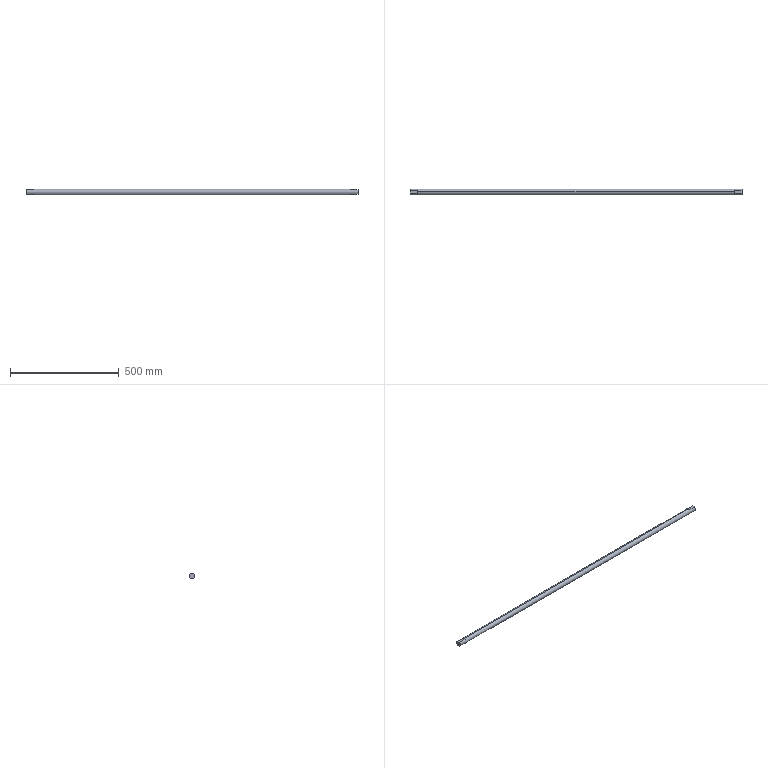Part | SolidWorks | features ICE 3, Extrusion 1, HoleWzd 1 | 1 solid | 12 faces | box 1530 x 25 x 25 mm | volume 749305 mm3 | plane 10 | cylinder 2 | commonest cylinder face diameters 25 x2
STEP:
#1=CARTESIAN_POINT('',(1494.,5.937,-11.));
#2=VERTEX_POINT('',#1);
#3=CARTESIAN_POINT('',(1494.,0.,-12.5));
#4=VERTEX_POINT('',#3);
#5=CARTESIAN_POINT('',(1494.,0.,0.));
#6=DIRECTION('',(-1.,0.,0.));
#7=DIRECTION('',(0.,0.,1.));
#8=AXIS2_PLACEMENT_3D('',#5,#6,#7);
#9=CIRCLE('',#8,12.5);
#10=EDGE_CURVE('',#2,#4,#9,.T.);
#11=ORIENTED_EDGE('',*,*,#10,.T.);
#12=CARTESIAN_POINT('',(36.,0.,-12.5));
#13=VERTEX_POINT('',#12);
#14=CARTESIAN_POINT('',(1530.,0.,-12.5));
#15=DIRECTION('',(-1.,0.,0.));
#16=VECTOR('',#15,1000.);
#17=LINE('',#14,#16);
#18=EDGE_CURVE('',#4,#13,#17,.T.);
#19=ORIENTED_EDGE('',*,*,#18,.T.);
#20=CARTESIAN_POINT('',(36.,5.937,-11.));
#21=VERTEX_POINT('',#20);
#22=CARTESIAN_POINT('',(36.,0.,0.));
#23=DIRECTION('',(1.,0.,0.));
#24=DIRECTION('',(0.,1.,0.));
#25=AXIS2_PLACEMENT_3D('',#22,#23,#24);
#26=CIRCLE('',#25,12.5);
#27=EDGE_CURVE('',#13,#21,#26,.T.);
#28=ORIENTED_EDGE('',*,*,#27,.T.);
#29=CARTESIAN_POINT('',(0.,5.937,-11.));
#30=VERTEX_POINT('',#29);
#31=CARTESIAN_POINT('',(1530.,5.937,-11.));
#32=DIRECTION('',(-1.,0.,0.));
#33=VECTOR('',#32,1000.);
#34=LINE('',#31,#33);
#35=EDGE_CURVE('',#21,#30,#34,.T.);
#36=ORIENTED_EDGE('',*,*,#35,.T.);
#37=CARTESIAN_POINT('',(0.,5.937,11.));
#38=VERTEX_POINT('',#37);
#39=CARTESIAN_POINT('',(0.,0.,0.));
#40=DIRECTION('',(1.,0.,0.));
#41=DIRECTION('',(0.,0.,-1.));
#42=AXIS2_PLACEMENT_3D('',#39,#40,#41);
#43=CIRCLE('',#42,12.5);
#44=EDGE_CURVE('',#30,#38,#43,.T.);
#45=ORIENTED_EDGE('',*,*,#44,.T.);
#46=CARTESIAN_POINT('',(36.,5.937,11.));
#47=VERTEX_POINT('',#46);
#48=CARTESIAN_POINT('',(1530.,5.937,11.));
#49=DIRECTION('',(-1.,0.,0.));
#50=VECTOR('',#49,1000.);
#51=LINE('',#48,#50);
#52=EDGE_CURVE('',#47,#38,#51,.T.);
#53=ORIENTED_EDGE('',*,*,#52,.F.);
#54=CARTESIAN_POINT('',(36.,0.,12.5));
#55=VERTEX_POINT('',#54);
#56=CARTESIAN_POINT('',(36.,0.,0.));
#57=DIRECTION('',(-1.,0.,0.));
#58=DIRECTION('',(0.,-1.,0.));
#59=AXIS2_PLACEMENT_3D('',#56,#57,#58);
#60=CIRCLE('',#59,12.5);
#61=EDGE_CURVE('',#55,#47,#60,.T.);
#62=ORIENTED_EDGE('',*,*,#61,.F.);
#63=CARTESIAN_POINT('',(1494.,0.,12.5));
#64=VERTEX_POINT('',#63);
#65=CARTESIAN_POINT('',(1530.,0.,12.5));
#66=DIRECTION('',(-1.,0.,0.));
#67=VECTOR('',#66,1000.);
#68=LINE('',#65,#67);
#69=EDGE_CURVE('',#64,#55,#68,.T.);
#70=ORIENTED_EDGE('',*,*,#69,.F.);
#71=CARTESIAN_POINT('',(1494.,5.937,11.));
#72=VERTEX_POINT('',#71);
#73=CARTESIAN_POINT('',(1494.,0.,0.));
#74=DIRECTION('',(1.,0.,0.));
#75=DIRECTION('',(0.,0.,-1.));
#76=AXIS2_PLACEMENT_3D('',#73,#74,#75);
#77=CIRCLE('',#76,12.5);
#78=EDGE_CURVE('',#72,#64,#77,.T.);
#79=ORIENTED_EDGE('',*,*,#78,.F.);
#80=CARTESIAN_POINT('',(1530.,5.937,11.));
#81=VERTEX_POINT('',#80);
#82=CARTESIAN_POINT('',(1530.,5.937,11.));
#83=DIRECTION('',(-1.,0.,0.));
#84=VECTOR('',#83,1000.);
#85=LINE('',#82,#84);
#86=EDGE_CURVE('',#81,#72,#85,.T.);
#87=ORIENTED_EDGE('',*,*,#86,.F.);
#88=CARTESIAN_POINT('',(1530.,5.937,-11.));
#89=VERTEX_POINT('',#88);
#90=CARTESIAN_POINT('',(1530.,0.,0.));
#91=DIRECTION('',(1.,0.,0.));
#92=DIRECTION('',(0.,0.,-1.));
#93=AXIS2_PLACEMENT_3D('',#90,#91,#92);
#94=CIRCLE('',#93,12.5);
#95=EDGE_CURVE('',#89,#81,#94,.T.);
#96=ORIENTED_EDGE('',*,*,#95,.F.);
#97=CARTESIAN_POINT('',(1530.,5.937,-11.));
#98=DIRECTION('',(-1.,0.,0.));
#99=VECTOR('',#98,1000.);
#100=LINE('',#97,#99);
#101=EDGE_CURVE('',#89,#2,#100,.T.);
#102=ORIENTED_EDGE('',*,*,#101,.T.);
#103=EDGE_LOOP('',(#11,#19,#28,#36,#45,#53,#62,#70,#79,#87,#96,#102));
#104=FACE_OUTER_BOUND('',#103,.T.);
#105=CARTESIAN_POINT('',(1530.,0.,0.));
#106=DIRECTION('',(-1.,0.,0.));
#107=DIRECTION('',(0.,0.,1.));
#108=AXIS2_PLACEMENT_3D('',#105,#106,#107);
#109=CYLINDRICAL_SURFACE('',#108,12.5);
#110=ADVANCED_FACE('',(#104),#109,.T.);
#111=ORIENTED_EDGE('',*,*,#18,.F.);
#112=CARTESIAN_POINT('',(1494.,-5.937,-11.));
#113=VERTEX_POINT('',#112);
#114=CARTESIAN_POINT('',(1494.,0.,0.));
#115=DIRECTION('',(-1.,0.,0.));
#116=DIRECTION('',(0.,0.,1.));
#117=AXIS2_PLACEMENT_3D('',#114,#115,#116);
#118=CIRCLE('',#117,12.5);
#119=EDGE_CURVE('',#4,#113,#118,.T.);
#120=ORIENTED_EDGE('',*,*,#119,.T.);
#121=CARTESIAN_POINT('',(1530.,-5.937,-11.));
#122=VERTEX_POINT('',#121);
#123=CARTESIAN_POINT('',(1530.,-5.937,-11.));
#124=DIRECTION('',(1.,0.,0.));
#125=VECTOR('',#124,1000.);
#126=LINE('',#123,#125);
#127=EDGE_CURVE('',#113,#122,#126,.T.);
#128=ORIENTED_EDGE('',*,*,#127,.T.);
#129=CARTESIAN_POINT('',(1530.,-5.937,11.));
#130=VERTEX_POINT('',#129);
#131=CARTESIAN_POINT('',(1530.,0.,0.));
#132=DIRECTION('',(1.,0.,0.));
#133=DIRECTION('',(0.,0.,-1.));
#134=AXIS2_PLACEMENT_3D('',#131,#132,#133);
#135=CIRCLE('',#134,12.5);
#136=EDGE_CURVE('',#130,#122,#135,.T.);
#137=ORIENTED_EDGE('',*,*,#136,.F.);
#138=CARTESIAN_POINT('',(1494.,-5.937,11.));
#139=VERTEX_POINT('',#138);
#140=CARTESIAN_POINT('',(1530.,-5.937,11.));
#141=DIRECTION('',(1.,0.,0.));
#142=VECTOR('',#141,1000.);
#143=LINE('',#140,#142);
#144=EDGE_CURVE('',#139,#130,#143,.T.);
#145=ORIENTED_EDGE('',*,*,#144,.F.);
#146=CARTESIAN_POINT('',(1494.,0.,0.));
#147=DIRECTION('',(1.,0.,0.));
#148=DIRECTION('',(0.,0.,-1.));
#149=AXIS2_PLACEMENT_3D('',#146,#147,#148);
#150=CIRCLE('',#149,12.5);
#151=EDGE_CURVE('',#64,#139,#150,.T.);
#152=ORIENTED_EDGE('',*,*,#151,.F.);
#153=ORIENTED_EDGE('',*,*,#69,.T.);
#154=CARTESIAN_POINT('',(36.,-5.937,11.));
#155=VERTEX_POINT('',#154);
#156=CARTESIAN_POINT('',(36.,0.,0.));
#157=DIRECTION('',(-1.,0.,0.));
#158=DIRECTION('',(0.,-1.,0.));
#159=AXIS2_PLACEMENT_3D('',#156,#157,#158);
#160=CIRCLE('',#159,12.5);
#161=EDGE_CURVE('',#155,#55,#160,.T.);
#162=ORIENTED_EDGE('',*,*,#161,.F.);
#163=CARTESIAN_POINT('',(0.,-5.937,11.));
#164=VERTEX_POINT('',#163);
#165=CARTESIAN_POINT('',(1530.,-5.937,11.));
#166=DIRECTION('',(1.,0.,0.));
#167=VECTOR('',#166,1000.);
#168=LINE('',#165,#167);
#169=EDGE_CURVE('',#164,#155,#168,.T.);
#170=ORIENTED_EDGE('',*,*,#169,.F.);
#171=CARTESIAN_POINT('',(0.,-5.937,-11.));
#172=VERTEX_POINT('',#171);
#173=CARTESIAN_POINT('',(0.,0.,0.));
#174=DIRECTION('',(1.,0.,0.));
#175=DIRECTION('',(0.,0.,-1.));
#176=AXIS2_PLACEMENT_3D('',#173,#174,#175);
#177=CIRCLE('',#176,12.5);
#178=EDGE_CURVE('',#164,#172,#177,.T.);
#179=ORIENTED_EDGE('',*,*,#178,.T.);
#180=CARTESIAN_POINT('',(36.,-5.937,-11.));
#181=VERTEX_POINT('',#180);
#182=CARTESIAN_POINT('',(1530.,-5.937,-11.));
#183=DIRECTION('',(1.,0.,0.));
#184=VECTOR('',#183,1000.);
#185=LINE('',#182,#184);
#186=EDGE_CURVE('',#172,#181,#185,.T.);
#187=ORIENTED_EDGE('',*,*,#186,.T.);
#188=CARTESIAN_POINT('',(36.,0.,0.));
#189=DIRECTION('',(1.,0.,0.));
#190=DIRECTION('',(0.,1.,0.));
#191=AXIS2_PLACEMENT_3D('',#188,#189,#190);
#192=CIRCLE('',#191,12.5);
#193=EDGE_CURVE('',#181,#13,#192,.T.);
#194=ORIENTED_EDGE('',*,*,#193,.T.);
#195=EDGE_LOOP('',(#111,#120,#128,#137,#145,#152,#153,#162,#170,#179,#187,#194));
#196=FACE_OUTER_BOUND('',#195,.T.);
#197=CARTESIAN_POINT('',(1530.,0.,0.));
#198=DIRECTION('',(-1.,0.,0.));
#199=DIRECTION('',(0.,0.,1.));
#200=AXIS2_PLACEMENT_3D('',#197,#198,#199);
#201=CYLINDRICAL_SURFACE('',#200,12.5);
#202=ADVANCED_FACE('',(#196),#201,.T.);
#203=ORIENTED_EDGE('',*,*,#95,.T.);
#204=CARTESIAN_POINT('',(1530.,0.,11.));
#205=DIRECTION('',(0.,-1.,0.));
#206=VECTOR('',#205,1000.);
#207=LINE('',#204,#206);
#208=EDGE_CURVE('',#81,#130,#207,.T.);
#209=ORIENTED_EDGE('',*,*,#208,.T.);
#210=ORIENTED_EDGE('',*,*,#136,.T.);
#211=CARTESIAN_POINT('',(1530.,0.,-11.));
#212=DIRECTION('',(0.,-1.,0.));
#213=VECTOR('',#212,1000.);
#214=LINE('',#211,#213);
#215=EDGE_CURVE('',#89,#122,#214,.T.);
#216=ORIENTED_EDGE('',*,*,#215,.F.);
#217=EDGE_LOOP('',(#203,#209,#210,#216));
#218=FACE_OUTER_BOUND('',#217,.T.);
#219=CARTESIAN_POINT('',(1530.,0.,0.));
#220=DIRECTION('',(1.,0.,0.));
#221=DIRECTION('',(0.,0.,-1.));
#222=AXIS2_PLACEMENT_3D('',#219,#220,#221);
#223=PLANE('',#222);
#224=ADVANCED_FACE('',(#218),#223,.T.);
#225=CARTESIAN_POINT('',(0.,0.,11.));
#226=DIRECTION('',(0.,-1.,0.));
#227=VECTOR('',#226,1000.);
#228=LINE('',#225,#227);
#229=EDGE_CURVE('',#38,#164,#228,.T.);
#230=ORIENTED_EDGE('',*,*,#229,.F.);
#231=ORIENTED_EDGE('',*,*,#44,.F.);
#232=CARTESIAN_POINT('',(0.,0.,-11.));
#233=DIRECTION('',(0.,-1.,0.));
#234=VECTOR('',#233,1000.);
#235=LINE('',#232,#234);
#236=EDGE_CURVE('',#30,#172,#235,.T.);
#237=ORIENTED_EDGE('',*,*,#236,.T.);
#238=ORIENTED_EDGE('',*,*,#178,.F.);
#239=EDGE_LOOP('',(#230,#231,#237,#238));
#240=FACE_OUTER_BOUND('',#239,.T.);
#241=CARTESIAN_POINT('',(0.,0.,0.));
#242=DIRECTION('',(1.,0.,0.));
#243=DIRECTION('',(0.,0.,-1.));
#244=AXIS2_PLACEMENT_3D('',#241,#242,#243);
#245=PLANE('',#244);
#246=ADVANCED_FACE('',(#240),#245,.F.);
#247=CARTESIAN_POINT('',(36.,29.983,-11.));
#248=DIRECTION('',(0.,1.,0.));
#249=VECTOR('',#248,1000.);
#250=LINE('',#247,#249);
#251=EDGE_CURVE('',#181,#21,#250,.T.);
#252=ORIENTED_EDGE('',*,*,#251,.T.);
#253=ORIENTED_EDGE('',*,*,#27,.F.);
#254=ORIENTED_EDGE('',*,*,#193,.F.);
#255=EDGE_LOOP('',(#252,#253,#254));
#256=FACE_OUTER_BOUND('',#255,.T.);
#257=CARTESIAN_POINT('',(36.,29.983,-31.));
#258=DIRECTION('',(1.,0.,0.));
#259=DIRECTION('',(0.,1.,0.));
#260=AXIS2_PLACEMENT_3D('',#257,#258,#259);
#261=PLANE('',#260);
#262=ADVANCED_FACE('',(#256),#261,.F.);
#263=ORIENTED_EDGE('',*,*,#251,.F.);
#264=ORIENTED_EDGE('',*,*,#186,.F.);
#265=ORIENTED_EDGE('',*,*,#236,.F.);
#266=ORIENTED_EDGE('',*,*,#35,.F.);
#267=EDGE_LOOP('',(#263,#264,#265,#266));
#268=FACE_OUTER_BOUND('',#267,.T.);
#269=CARTESIAN_POINT('',(0.,0.,-11.));
#270=DIRECTION('',(0.,0.,1.));
#271=DIRECTION('',(1.,0.,0.));
#272=AXIS2_PLACEMENT_3D('',#269,#270,#271);
#273=PLANE('',#272);
#274=ADVANCED_FACE('',(#268),#273,.F.);
#275=CARTESIAN_POINT('',(1494.,29.983,-11.));
#276=DIRECTION('',(0.,-1.,0.));
#277=VECTOR('',#276,1000.);
#278=LINE('',#275,#277);
#279=EDGE_CURVE('',#2,#113,#278,.T.);
#280=ORIENTED_EDGE('',*,*,#279,.T.);
#281=ORIENTED_EDGE('',*,*,#119,.F.);
#282=ORIENTED_EDGE('',*,*,#10,.F.);
#283=EDGE_LOOP('',(#280,#281,#282));
#284=FACE_OUTER_BOUND('',#283,.T.);
#285=CARTESIAN_POINT('',(1494.,29.983,-31.));
#286=DIRECTION('',(-1.,0.,0.));
#287=DIRECTION('',(0.,0.,1.));
#288=AXIS2_PLACEMENT_3D('',#285,#286,#287);
#289=PLANE('',#288);
#290=ADVANCED_FACE('',(#284),#289,.F.);
#291=ORIENTED_EDGE('',*,*,#215,.T.);
#292=ORIENTED_EDGE('',*,*,#127,.F.);
#293=ORIENTED_EDGE('',*,*,#279,.F.);
#294=ORIENTED_EDGE('',*,*,#101,.F.);
#295=EDGE_LOOP('',(#291,#292,#293,#294));
#296=FACE_OUTER_BOUND('',#295,.T.);
#297=CARTESIAN_POINT('',(0.,0.,-11.));
#298=DIRECTION('',(0.,0.,1.));
#299=DIRECTION('',(1.,0.,0.));
#300=AXIS2_PLACEMENT_3D('',#297,#298,#299);
#301=PLANE('',#300);
#302=ADVANCED_FACE('',(#296),#301,.F.);
#303=ORIENTED_EDGE('',*,*,#161,.T.);
#304=ORIENTED_EDGE('',*,*,#61,.T.);
#305=CARTESIAN_POINT('',(36.,29.983,11.));
#306=DIRECTION('',(0.,1.,0.));
#307=VECTOR('',#306,1000.);
#308=LINE('',#305,#307);
#309=EDGE_CURVE('',#155,#47,#308,.T.);
#310=ORIENTED_EDGE('',*,*,#309,.F.);
#311=EDGE_LOOP('',(#303,#304,#310));
#312=FACE_OUTER_BOUND('',#311,.T.);
#313=CARTESIAN_POINT('',(36.,29.983,31.));
#314=DIRECTION('',(-1.,0.,0.));
#315=DIRECTION('',(0.,-1.,0.));
#316=AXIS2_PLACEMENT_3D('',#313,#314,#315);
#317=PLANE('',#316);
#318=ADVANCED_FACE('',(#312),#317,.T.);
#319=ORIENTED_EDGE('',*,*,#52,.T.);
#320=ORIENTED_EDGE('',*,*,#229,.T.);
#321=ORIENTED_EDGE('',*,*,#169,.T.);
#322=ORIENTED_EDGE('',*,*,#309,.T.);
#323=EDGE_LOOP('',(#319,#320,#321,#322));
#324=FACE_OUTER_BOUND('',#323,.T.);
#325=CARTESIAN_POINT('',(0.,0.,11.));
#326=DIRECTION('',(0.,0.,1.));
#327=DIRECTION('',(1.,0.,0.));
#328=AXIS2_PLACEMENT_3D('',#325,#326,#327);
#329=PLANE('',#328);
#330=ADVANCED_FACE('',(#324),#329,.T.);
#331=ORIENTED_EDGE('',*,*,#78,.T.);
#332=ORIENTED_EDGE('',*,*,#151,.T.);
#333=CARTESIAN_POINT('',(1494.,29.983,11.));
#334=DIRECTION('',(0.,-1.,0.));
#335=VECTOR('',#334,1000.);
#336=LINE('',#333,#335);
#337=EDGE_CURVE('',#72,#139,#336,.T.);
#338=ORIENTED_EDGE('',*,*,#337,.F.);
#339=EDGE_LOOP('',(#331,#332,#338));
#340=FACE_OUTER_BOUND('',#339,.T.);
#341=CARTESIAN_POINT('',(1494.,29.983,31.));
#342=DIRECTION('',(1.,0.,0.));
#343=DIRECTION('',(0.,0.,-1.));
#344=AXIS2_PLACEMENT_3D('',#341,#342,#343);
#345=PLANE('',#344);
#346=ADVANCED_FACE('',(#340),#345,.T.);
#347=ORIENTED_EDGE('',*,*,#86,.T.);
#348=ORIENTED_EDGE('',*,*,#337,.T.);
#349=ORIENTED_EDGE('',*,*,#144,.T.);
#350=ORIENTED_EDGE('',*,*,#208,.F.);
#351=EDGE_LOOP('',(#347,#348,#349,#350));
#352=FACE_OUTER_BOUND('',#351,.T.);
#353=CARTESIAN_POINT('',(0.,0.,11.));
#354=DIRECTION('',(0.,0.,1.));
#355=DIRECTION('',(1.,0.,0.));
#356=AXIS2_PLACEMENT_3D('',#353,#354,#355);
#357=PLANE('',#356);
#358=ADVANCED_FACE('',(#352),#357,.T.);
#359=CLOSED_SHELL('',(#110,#202,#224,#246,#262,#274,#290,#302,#318,#330,#346,#358));
#360=MANIFOLD_SOLID_BREP('',#359);
#361=CARTESIAN_POINT('',(0.,0.,0.));
#362=DIRECTION('',(0.,0.,1.));
#363=DIRECTION('',(1.,0.,0.));
#364=AXIS2_PLACEMENT_3D('',#361,#362,#363);
#365=(LENGTH_UNIT()NAMED_UNIT(*)SI_UNIT(.MILLI.,.METRE.));
#366=UNCERTAINTY_MEASURE_WITH_UNIT(LENGTH_MEASURE(0.00001),#365,'','');
#367=(NAMED_UNIT(*)PLANE_ANGLE_UNIT()SI_UNIT($,.RADIAN.));
#368=(NAMED_UNIT(*)SI_UNIT($,.STERADIAN.)SOLID_ANGLE_UNIT());
#369=(GEOMETRIC_REPRESENTATION_CONTEXT(3)GLOBAL_UNCERTAINTY_ASSIGNED_CONTEXT((#366))GLOBAL_UNIT_ASSIGNED_CONTEXT((#365,#367,#368))REPRESENTATION_CONTEXT('',''));
#370=ADVANCED_BREP_SHAPE_REPRESENTATION('',(#360,#364),#369);